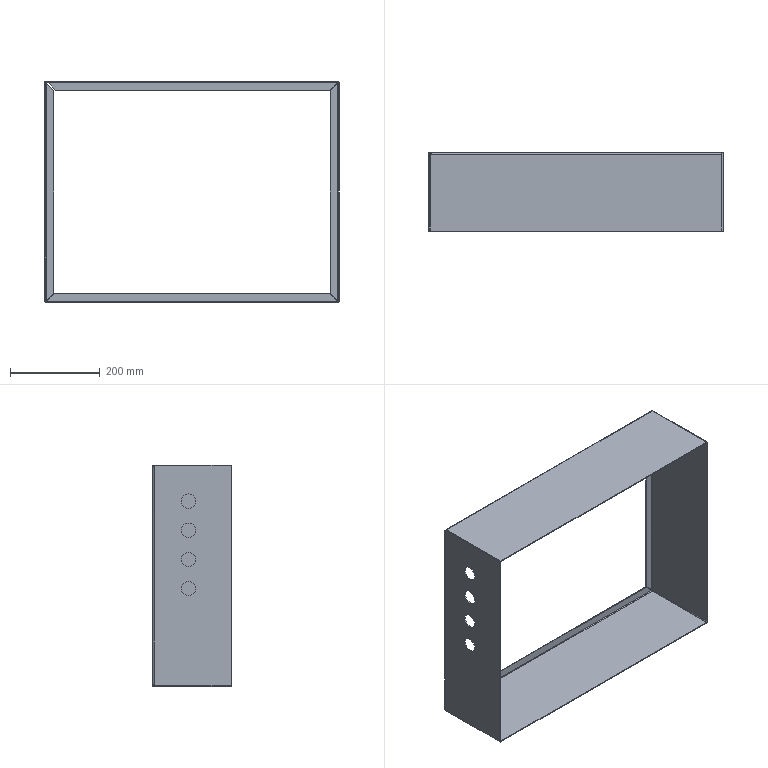Part | STEP file | Distribution box body SGN-1-12-01 | 1 solid | 76 faces | box 656 x 175 x 494 mm | volume 868772 mm3 | plane 46 | cylinder 22 | spline 8 | commonest cylinder face diameters 32 x8 3 x7 7 x7